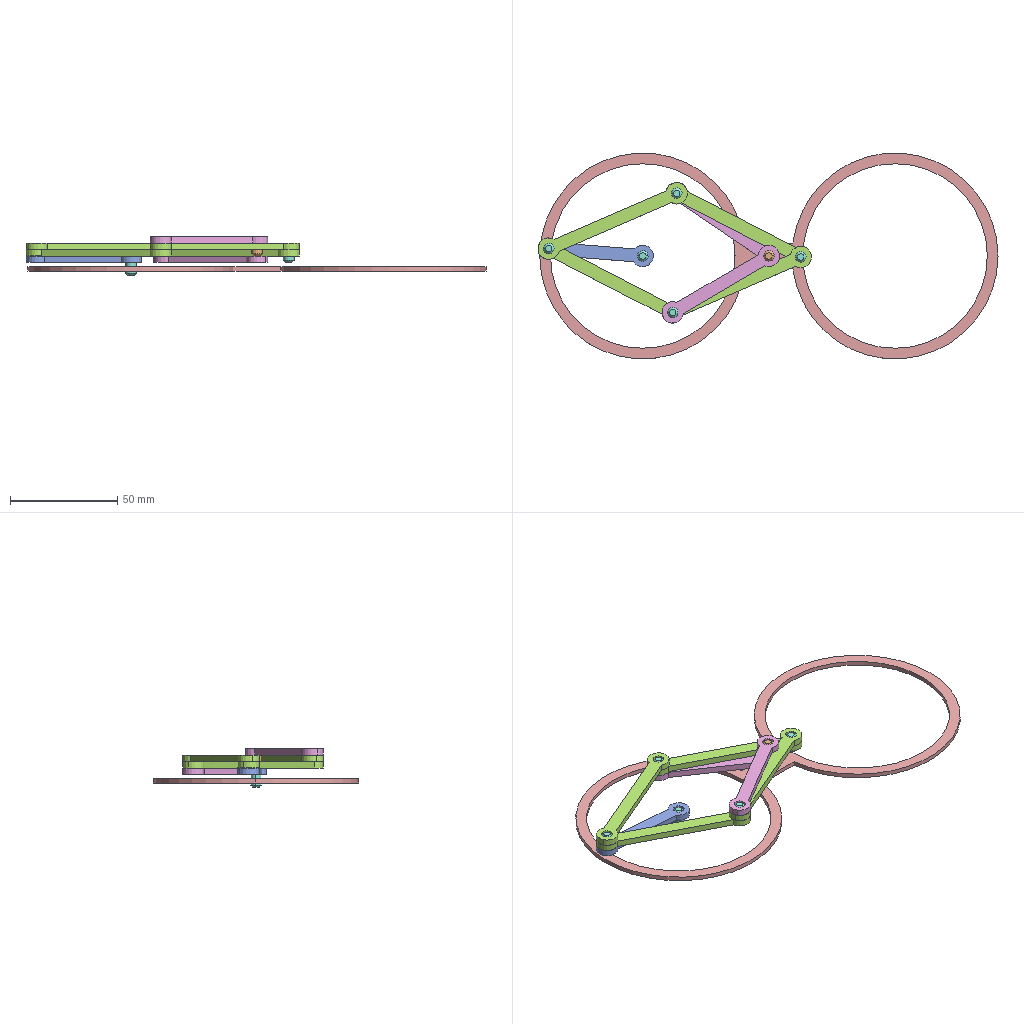Assembly | SolidWorks | 6 different items | 14 placed | box 214 x 96 x 18 mm
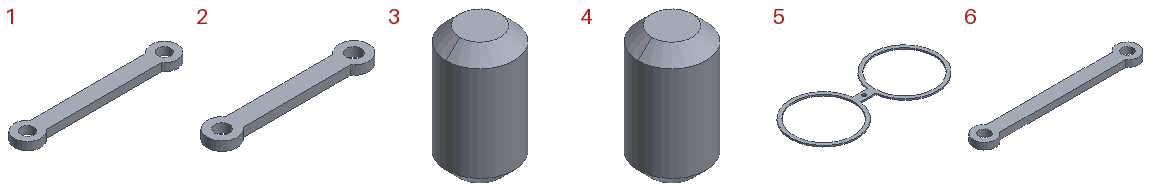Parts list (item | quantity | size | volume | features):
1 | x2 | 62 x 10 x 3 mm | 1121 mm3 | features Extrusion 1
2 | x1 | 54 x 10 x 3 mm | 976.904 mm3 | features Extrusion 1
3 | x5 | 5 x 5 x 9 mm | 163.101 mm3 | features Chamfer 1, Extrusion 1
4 | x1 | 5 x 5 x 9 mm | 163.101 mm3 | features Chamfer 1, Extrusion 1
5 | x1 | 213.58 x 96 x 2 mm | 6205 mm3 | features Extrusion 1
6 | x4 | 75 x 10 x 3 mm | 1355 mm3 | features Extrusion 1
Mates (type | each side: item.copy, entity, surface, feature):
Concentric | 5.1 face cylinder Boss-Extrude1 | 2.1 face cylinder Boss-Extrude1
Concentric | 6.1 face cylinder Boss-Extrude1 | 6.2 face cylinder Boss-Extrude1
Concentric | 6.3 face cylinder Boss-Extrude1 | 6.2 face cylinder Boss-Extrude1
Concentric | 6.3 face cylinder Boss-Extrude1 | 6.4 face cylinder Boss-Extrude1
Concentric | 6.1 face cylinder Boss-Extrude1 | 6.4 face cylinder Boss-Extrude1
Concentric | 6.2 face cylinder Boss-Extrude1 | 1.1 face cylinder Boss-Extrude1
Concentric | 1.2 face cylinder Boss-Extrude1 | 1.1 face cylinder Boss-Extrude1
Concentric | 6.4 face cylinder Boss-Extrude1 | 1.2 face cylinder Boss-Extrude1
Coincident | 6.1 face plane Boss-Extrude1 | 6.2 face plane Boss-Extrude1
Concentric | 5.1 face cylinder Boss-Extrude1 | 1.2 face cylinder Boss-Extrude1
Concentric | 2.1 face cylinder Boss-Extrude1 | 6.1 face cylinder Boss-Extrude1
DistanceDim | 6.4 face plane Boss-Extrude1 | 5.1 face plane Boss-Extrude1
Coincident | 6.3 face plane Boss-Extrude1 | 6.4 face plane Boss-Extrude1
Coincident | 6.4 face plane Boss-Extrude1 | 1.2 face plane Boss-Extrude1
Coincident | 6.1 face plane Boss-Extrude1 | 1.1 face plane Boss-Extrude1
Coincident | 6.3 face plane Boss-Extrude1 | 6.2 face plane Boss-Extrude1
Coincident | 2.1 face plane Boss-Extrude1 | 6.2 face plane Boss-Extrude1
Concentric | 6.1 face cylinder Boss-Extrude1 | 3.1 face cylinder Boss-Extrude1
Coincident | 6.1 face plane Boss-Extrude1 | 3.1 face plane Boss-Extrude1
Concentric | 1.1 face cylinder Boss-Extrude1 | 3.2 face cylinder Boss-Extrude1
Coincident | 1.1 face plane Boss-Extrude1 | 3.2 face plane Boss-Extrude1
Concentric | 6.1 face cylinder Boss-Extrude1 | 3.3 face cylinder Boss-Extrude1
Coincident | 6.1 face plane Boss-Extrude1 | 3.3 face plane Boss-Extrude1
Concentric | 2.1 face cylinder Boss-Extrude1 | 3.4 face cylinder Boss-Extrude1
Coincident | 2.1 face plane Boss-Extrude1 | 3.4 face plane Boss-Extrude1
Concentric | 6.3 face cylinder Boss-Extrude1 | 3.5 face cylinder Boss-Extrude1
Coincident | 6.3 face plane Boss-Extrude1 | 3.5 face plane Boss-Extrude1
Concentric | 1.1 face cylinder Boss-Extrude1 | 4.1 face cylinder Boss-Extrude1
Coincident | 1.1 face plane Boss-Extrude1 | 4.1 face plane Boss-Extrude1